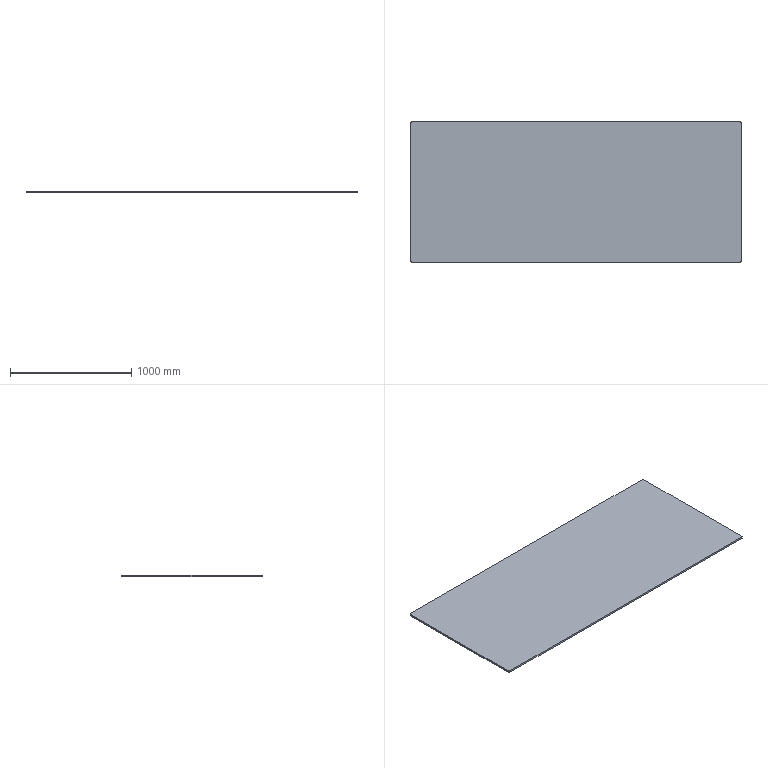Part | STEP file | Part 6 | 1 solid | 10 faces | box 2720 x 1160 x 15 mm | volume 47326712 mm3 | plane 6 | cylinder 4 | commonest cylinder face diameters 20 x4
STEP:
#1=CARTESIAN_POINT('',(1360.,-570.,0.));
#2=VERTEX_POINT('',#1);
#3=CARTESIAN_POINT('',(1360.,570.,0.));
#4=VERTEX_POINT('',#3);
#5=CARTESIAN_POINT('',(1360.,580.,0.));
#6=DIRECTION('',(0.,1.,0.));
#7=VECTOR('',#6,1000.);
#8=LINE('',#5,#7);
#9=EDGE_CURVE('',#2,#4,#8,.T.);
#10=ORIENTED_EDGE('',*,*,#9,.T.);
#11=CARTESIAN_POINT('',(1360.,570.,15.));
#12=VERTEX_POINT('',#11);
#13=CARTESIAN_POINT('',(1360.,570.,15.));
#14=DIRECTION('',(0.,0.,1.));
#15=VECTOR('',#14,1000.);
#16=LINE('',#13,#15);
#17=EDGE_CURVE('',#4,#12,#16,.T.);
#18=ORIENTED_EDGE('',*,*,#17,.T.);
#19=CARTESIAN_POINT('',(1360.,-570.,15.));
#20=VERTEX_POINT('',#19);
#21=CARTESIAN_POINT('',(1360.,580.,15.));
#22=DIRECTION('',(0.,1.,0.));
#23=VECTOR('',#22,1000.);
#24=LINE('',#21,#23);
#25=EDGE_CURVE('',#20,#12,#24,.T.);
#26=ORIENTED_EDGE('',*,*,#25,.F.);
#27=CARTESIAN_POINT('',(1360.,-570.,15.));
#28=DIRECTION('',(0.,0.,-1.));
#29=VECTOR('',#28,1000.);
#30=LINE('',#27,#29);
#31=EDGE_CURVE('',#20,#2,#30,.T.);
#32=ORIENTED_EDGE('',*,*,#31,.T.);
#33=EDGE_LOOP('',(#10,#18,#26,#32));
#34=FACE_OUTER_BOUND('',#33,.T.);
#35=CARTESIAN_POINT('',(1360.,580.,15.));
#36=DIRECTION('',(-1.,0.,0.));
#37=DIRECTION('',(0.,-1.,0.));
#38=AXIS2_PLACEMENT_3D('',#35,#36,#37);
#39=PLANE('',#38);
#40=ADVANCED_FACE('',(#34),#39,.F.);
#41=CARTESIAN_POINT('',(1350.,580.,15.));
#42=VERTEX_POINT('',#41);
#43=CARTESIAN_POINT('',(-1350.,580.,15.));
#44=VERTEX_POINT('',#43);
#45=CARTESIAN_POINT('',(-1360.,580.,15.));
#46=DIRECTION('',(-1.,0.,0.));
#47=VECTOR('',#46,1000.);
#48=LINE('',#45,#47);
#49=EDGE_CURVE('',#42,#44,#48,.T.);
#50=ORIENTED_EDGE('',*,*,#49,.F.);
#51=CARTESIAN_POINT('',(1350.,580.,0.));
#52=VERTEX_POINT('',#51);
#53=CARTESIAN_POINT('',(1350.,580.,15.));
#54=DIRECTION('',(0.,0.,-1.));
#55=VECTOR('',#54,1000.);
#56=LINE('',#53,#55);
#57=EDGE_CURVE('',#42,#52,#56,.T.);
#58=ORIENTED_EDGE('',*,*,#57,.T.);
#59=CARTESIAN_POINT('',(-1350.,580.,0.));
#60=VERTEX_POINT('',#59);
#61=CARTESIAN_POINT('',(-1360.,580.,0.));
#62=DIRECTION('',(-1.,0.,0.));
#63=VECTOR('',#62,1000.);
#64=LINE('',#61,#63);
#65=EDGE_CURVE('',#52,#60,#64,.T.);
#66=ORIENTED_EDGE('',*,*,#65,.T.);
#67=CARTESIAN_POINT('',(-1350.,580.,15.));
#68=DIRECTION('',(0.,0.,1.));
#69=VECTOR('',#68,1000.);
#70=LINE('',#67,#69);
#71=EDGE_CURVE('',#60,#44,#70,.T.);
#72=ORIENTED_EDGE('',*,*,#71,.T.);
#73=EDGE_LOOP('',(#50,#58,#66,#72));
#74=FACE_OUTER_BOUND('',#73,.T.);
#75=CARTESIAN_POINT('',(-1360.,580.,15.));
#76=DIRECTION('',(0.,-1.,0.));
#77=DIRECTION('',(1.,0.,0.));
#78=AXIS2_PLACEMENT_3D('',#75,#76,#77);
#79=PLANE('',#78);
#80=ADVANCED_FACE('',(#74),#79,.F.);
#81=CARTESIAN_POINT('',(-1360.,570.,0.));
#82=VERTEX_POINT('',#81);
#83=CARTESIAN_POINT('',(-1360.,-570.,0.));
#84=VERTEX_POINT('',#83);
#85=CARTESIAN_POINT('',(-1360.,580.,0.));
#86=DIRECTION('',(0.,-1.,0.));
#87=VECTOR('',#86,1000.);
#88=LINE('',#85,#87);
#89=EDGE_CURVE('',#82,#84,#88,.T.);
#90=ORIENTED_EDGE('',*,*,#89,.T.);
#91=CARTESIAN_POINT('',(-1360.,-570.,15.));
#92=VERTEX_POINT('',#91);
#93=CARTESIAN_POINT('',(-1360.,-570.,15.));
#94=DIRECTION('',(0.,0.,1.));
#95=VECTOR('',#94,1000.);
#96=LINE('',#93,#95);
#97=EDGE_CURVE('',#84,#92,#96,.T.);
#98=ORIENTED_EDGE('',*,*,#97,.T.);
#99=CARTESIAN_POINT('',(-1360.,570.,15.));
#100=VERTEX_POINT('',#99);
#101=CARTESIAN_POINT('',(-1360.,580.,15.));
#102=DIRECTION('',(0.,-1.,0.));
#103=VECTOR('',#102,1000.);
#104=LINE('',#101,#103);
#105=EDGE_CURVE('',#100,#92,#104,.T.);
#106=ORIENTED_EDGE('',*,*,#105,.F.);
#107=CARTESIAN_POINT('',(-1360.,570.,15.));
#108=DIRECTION('',(0.,0.,-1.));
#109=VECTOR('',#108,1000.);
#110=LINE('',#107,#109);
#111=EDGE_CURVE('',#100,#82,#110,.T.);
#112=ORIENTED_EDGE('',*,*,#111,.T.);
#113=EDGE_LOOP('',(#90,#98,#106,#112));
#114=FACE_OUTER_BOUND('',#113,.T.);
#115=CARTESIAN_POINT('',(-1360.,580.,15.));
#116=DIRECTION('',(1.,0.,0.));
#117=DIRECTION('',(0.,1.,0.));
#118=AXIS2_PLACEMENT_3D('',#115,#116,#117);
#119=PLANE('',#118);
#120=ADVANCED_FACE('',(#114),#119,.F.);
#121=CARTESIAN_POINT('',(-1350.,-580.,0.));
#122=VERTEX_POINT('',#121);
#123=CARTESIAN_POINT('',(1350.,-580.,0.));
#124=VERTEX_POINT('',#123);
#125=CARTESIAN_POINT('',(-1360.,-580.,0.));
#126=DIRECTION('',(1.,0.,0.));
#127=VECTOR('',#126,1000.);
#128=LINE('',#125,#127);
#129=EDGE_CURVE('',#122,#124,#128,.T.);
#130=ORIENTED_EDGE('',*,*,#129,.T.);
#131=CARTESIAN_POINT('',(1350.,-580.,15.));
#132=VERTEX_POINT('',#131);
#133=CARTESIAN_POINT('',(1350.,-580.,15.));
#134=DIRECTION('',(0.,0.,1.));
#135=VECTOR('',#134,1000.);
#136=LINE('',#133,#135);
#137=EDGE_CURVE('',#124,#132,#136,.T.);
#138=ORIENTED_EDGE('',*,*,#137,.T.);
#139=CARTESIAN_POINT('',(-1350.,-580.,15.));
#140=VERTEX_POINT('',#139);
#141=CARTESIAN_POINT('',(-1360.,-580.,15.));
#142=DIRECTION('',(1.,0.,0.));
#143=VECTOR('',#142,1000.);
#144=LINE('',#141,#143);
#145=EDGE_CURVE('',#140,#132,#144,.T.);
#146=ORIENTED_EDGE('',*,*,#145,.F.);
#147=CARTESIAN_POINT('',(-1350.,-580.,15.));
#148=DIRECTION('',(0.,0.,-1.));
#149=VECTOR('',#148,1000.);
#150=LINE('',#147,#149);
#151=EDGE_CURVE('',#140,#122,#150,.T.);
#152=ORIENTED_EDGE('',*,*,#151,.T.);
#153=EDGE_LOOP('',(#130,#138,#146,#152));
#154=FACE_OUTER_BOUND('',#153,.T.);
#155=CARTESIAN_POINT('',(-1360.,-580.,15.));
#156=DIRECTION('',(0.,1.,0.));
#157=DIRECTION('',(0.,0.,1.));
#158=AXIS2_PLACEMENT_3D('',#155,#156,#157);
#159=PLANE('',#158);
#160=ADVANCED_FACE('',(#154),#159,.F.);
#161=ORIENTED_EDGE('',*,*,#25,.T.);
#162=CARTESIAN_POINT('',(1350.,570.,15.));
#163=DIRECTION('',(0.,0.,1.));
#164=DIRECTION('',(1.,0.,0.));
#165=AXIS2_PLACEMENT_3D('',#162,#163,#164);
#166=CIRCLE('',#165,10.);
#167=EDGE_CURVE('',#12,#42,#166,.T.);
#168=ORIENTED_EDGE('',*,*,#167,.T.);
#169=ORIENTED_EDGE('',*,*,#49,.T.);
#170=CARTESIAN_POINT('',(-1350.,570.,15.));
#171=DIRECTION('',(0.,0.,1.));
#172=DIRECTION('',(1.,0.,0.));
#173=AXIS2_PLACEMENT_3D('',#170,#171,#172);
#174=CIRCLE('',#173,10.);
#175=EDGE_CURVE('',#44,#100,#174,.T.);
#176=ORIENTED_EDGE('',*,*,#175,.T.);
#177=ORIENTED_EDGE('',*,*,#105,.T.);
#178=CARTESIAN_POINT('',(-1350.,-570.,15.));
#179=DIRECTION('',(0.,0.,1.));
#180=DIRECTION('',(1.,0.,0.));
#181=AXIS2_PLACEMENT_3D('',#178,#179,#180);
#182=CIRCLE('',#181,10.);
#183=EDGE_CURVE('',#92,#140,#182,.T.);
#184=ORIENTED_EDGE('',*,*,#183,.T.);
#185=ORIENTED_EDGE('',*,*,#145,.T.);
#186=CARTESIAN_POINT('',(1350.,-570.,15.));
#187=DIRECTION('',(0.,0.,1.));
#188=DIRECTION('',(1.,0.,0.));
#189=AXIS2_PLACEMENT_3D('',#186,#187,#188);
#190=CIRCLE('',#189,10.);
#191=EDGE_CURVE('',#132,#20,#190,.T.);
#192=ORIENTED_EDGE('',*,*,#191,.T.);
#193=EDGE_LOOP('',(#161,#168,#169,#176,#177,#184,#185,#192));
#194=FACE_OUTER_BOUND('',#193,.T.);
#195=CARTESIAN_POINT('',(0.,0.,15.));
#196=DIRECTION('',(0.,0.,1.));
#197=DIRECTION('',(1.,0.,0.));
#198=AXIS2_PLACEMENT_3D('',#195,#196,#197);
#199=PLANE('',#198);
#200=ADVANCED_FACE('',(#194),#199,.T.);
#201=ORIENTED_EDGE('',*,*,#65,.F.);
#202=CARTESIAN_POINT('',(1350.,570.,0.));
#203=DIRECTION('',(0.,0.,-1.));
#204=DIRECTION('',(1.,0.,0.));
#205=AXIS2_PLACEMENT_3D('',#202,#203,#204);
#206=CIRCLE('',#205,10.);
#207=EDGE_CURVE('',#52,#4,#206,.T.);
#208=ORIENTED_EDGE('',*,*,#207,.T.);
#209=ORIENTED_EDGE('',*,*,#9,.F.);
#210=CARTESIAN_POINT('',(1350.,-570.,0.));
#211=DIRECTION('',(0.,0.,-1.));
#212=DIRECTION('',(1.,0.,0.));
#213=AXIS2_PLACEMENT_3D('',#210,#211,#212);
#214=CIRCLE('',#213,10.);
#215=EDGE_CURVE('',#2,#124,#214,.T.);
#216=ORIENTED_EDGE('',*,*,#215,.T.);
#217=ORIENTED_EDGE('',*,*,#129,.F.);
#218=CARTESIAN_POINT('',(-1350.,-570.,0.));
#219=DIRECTION('',(0.,0.,-1.));
#220=DIRECTION('',(1.,0.,0.));
#221=AXIS2_PLACEMENT_3D('',#218,#219,#220);
#222=CIRCLE('',#221,10.);
#223=EDGE_CURVE('',#122,#84,#222,.T.);
#224=ORIENTED_EDGE('',*,*,#223,.T.);
#225=ORIENTED_EDGE('',*,*,#89,.F.);
#226=CARTESIAN_POINT('',(-1350.,570.,0.));
#227=DIRECTION('',(0.,0.,-1.));
#228=DIRECTION('',(1.,0.,0.));
#229=AXIS2_PLACEMENT_3D('',#226,#227,#228);
#230=CIRCLE('',#229,10.);
#231=EDGE_CURVE('',#82,#60,#230,.T.);
#232=ORIENTED_EDGE('',*,*,#231,.T.);
#233=EDGE_LOOP('',(#201,#208,#209,#216,#217,#224,#225,#232));
#234=FACE_OUTER_BOUND('',#233,.T.);
#235=CARTESIAN_POINT('',(0.,0.,0.));
#236=DIRECTION('',(0.,0.,1.));
#237=DIRECTION('',(1.,0.,0.));
#238=AXIS2_PLACEMENT_3D('',#235,#236,#237);
#239=PLANE('',#238);
#240=ADVANCED_FACE('',(#234),#239,.F.);
#241=ORIENTED_EDGE('',*,*,#167,.F.);
#242=ORIENTED_EDGE('',*,*,#17,.F.);
#243=ORIENTED_EDGE('',*,*,#207,.F.);
#244=ORIENTED_EDGE('',*,*,#57,.F.);
#245=EDGE_LOOP('',(#241,#242,#243,#244));
#246=FACE_OUTER_BOUND('',#245,.T.);
#247=CARTESIAN_POINT('',(1350.,570.,15.));
#248=DIRECTION('',(0.,0.,-1.));
#249=DIRECTION('',(-1.,0.,0.));
#250=AXIS2_PLACEMENT_3D('',#247,#248,#249);
#251=CYLINDRICAL_SURFACE('',#250,10.);
#252=ADVANCED_FACE('',(#246),#251,.T.);
#253=ORIENTED_EDGE('',*,*,#191,.F.);
#254=ORIENTED_EDGE('',*,*,#137,.F.);
#255=ORIENTED_EDGE('',*,*,#215,.F.);
#256=ORIENTED_EDGE('',*,*,#31,.F.);
#257=EDGE_LOOP('',(#253,#254,#255,#256));
#258=FACE_OUTER_BOUND('',#257,.T.);
#259=CARTESIAN_POINT('',(1350.,-570.,15.));
#260=DIRECTION('',(0.,0.,-1.));
#261=DIRECTION('',(-1.,0.,0.));
#262=AXIS2_PLACEMENT_3D('',#259,#260,#261);
#263=CYLINDRICAL_SURFACE('',#262,10.);
#264=ADVANCED_FACE('',(#258),#263,.T.);
#265=ORIENTED_EDGE('',*,*,#183,.F.);
#266=ORIENTED_EDGE('',*,*,#97,.F.);
#267=ORIENTED_EDGE('',*,*,#223,.F.);
#268=ORIENTED_EDGE('',*,*,#151,.F.);
#269=EDGE_LOOP('',(#265,#266,#267,#268));
#270=FACE_OUTER_BOUND('',#269,.T.);
#271=CARTESIAN_POINT('',(-1350.,-570.,15.));
#272=DIRECTION('',(0.,0.,-1.));
#273=DIRECTION('',(-1.,0.,0.));
#274=AXIS2_PLACEMENT_3D('',#271,#272,#273);
#275=CYLINDRICAL_SURFACE('',#274,10.);
#276=ADVANCED_FACE('',(#270),#275,.T.);
#277=ORIENTED_EDGE('',*,*,#175,.F.);
#278=ORIENTED_EDGE('',*,*,#71,.F.);
#279=ORIENTED_EDGE('',*,*,#231,.F.);
#280=ORIENTED_EDGE('',*,*,#111,.F.);
#281=EDGE_LOOP('',(#277,#278,#279,#280));
#282=FACE_OUTER_BOUND('',#281,.T.);
#283=CARTESIAN_POINT('',(-1350.,570.,15.));
#284=DIRECTION('',(0.,0.,-1.));
#285=DIRECTION('',(-1.,0.,0.));
#286=AXIS2_PLACEMENT_3D('',#283,#284,#285);
#287=CYLINDRICAL_SURFACE('',#286,10.);
#288=ADVANCED_FACE('',(#282),#287,.T.);
#289=CLOSED_SHELL('',(#40,#80,#120,#160,#200,#240,#252,#264,#276,#288));
#290=MANIFOLD_SOLID_BREP('',#289);
#291=CARTESIAN_POINT('',(0.,0.,0.));
#292=DIRECTION('',(0.,0.,1.));
#293=DIRECTION('',(1.,0.,0.));
#294=AXIS2_PLACEMENT_3D('',#291,#292,#293);
#295=(LENGTH_UNIT()NAMED_UNIT(*)SI_UNIT(.MILLI.,.METRE.));
#296=UNCERTAINTY_MEASURE_WITH_UNIT(LENGTH_MEASURE(0.00001),#295,'','');
#297=(NAMED_UNIT(*)PLANE_ANGLE_UNIT()SI_UNIT($,.RADIAN.));
#298=(NAMED_UNIT(*)SI_UNIT($,.STERADIAN.)SOLID_ANGLE_UNIT());
#299=(GEOMETRIC_REPRESENTATION_CONTEXT(3)GLOBAL_UNCERTAINTY_ASSIGNED_CONTEXT((#296))GLOBAL_UNIT_ASSIGNED_CONTEXT((#295,#297,#298))REPRESENTATION_CONTEXT('',''));
#300=ADVANCED_BREP_SHAPE_REPRESENTATION('',(#290,#294),#299);